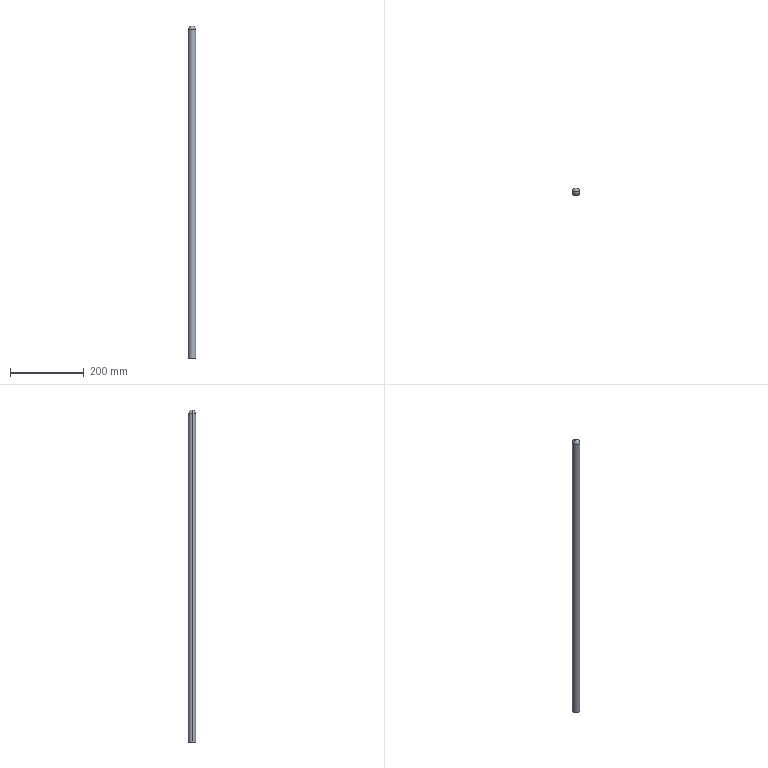Part | STEP file | X77-09003h | 1 solid | 6 faces | box 20 x 20 x 900 mm | volume 281698 mm3 | torus 2 | cylinder 2 | plane 2 | commonest cylinder face diameters 20 x2
STEP:
#1=CARTESIAN_POINT('',(-10.,0.,890.01));
#2=VERTEX_POINT('',#1);
#3=CARTESIAN_POINT('',(10.,0.,890.01));
#4=VERTEX_POINT('',#3);
#5=CARTESIAN_POINT('',(0.,0.,890.01));
#6=DIRECTION('',(0.,0.,-1.));
#7=DIRECTION('',(1.,0.,0.));
#8=AXIS2_PLACEMENT_3D('',#5,#6,#7);
#9=CIRCLE('',#8,10.);
#10=EDGE_CURVE('',#2,#4,#9,.T.);
#11=ORIENTED_EDGE('',*,*,#10,.F.);
#12=CARTESIAN_POINT('',(-0.01,0.,900.));
#13=VERTEX_POINT('',#12);
#14=CARTESIAN_POINT('',(-0.01,0.,890.01));
#15=DIRECTION('',(0.,1.,0.));
#16=DIRECTION('',(-1.,0.,0.));
#17=AXIS2_PLACEMENT_3D('',#14,#15,#16);
#18=CIRCLE('',#17,9.99);
#19=EDGE_CURVE('',#2,#13,#18,.T.);
#20=ORIENTED_EDGE('',*,*,#19,.T.);
#21=CARTESIAN_POINT('',(0.01,0.,900.));
#22=VERTEX_POINT('',#21);
#23=CARTESIAN_POINT('',(0.,0.,900.));
#24=DIRECTION('',(0.,0.,1.));
#25=DIRECTION('',(1.,0.,0.));
#26=AXIS2_PLACEMENT_3D('',#23,#24,#25);
#27=CIRCLE('',#26,0.01);
#28=EDGE_CURVE('',#22,#13,#27,.T.);
#29=ORIENTED_EDGE('',*,*,#28,.F.);
#30=CARTESIAN_POINT('',(0.01,0.,890.01));
#31=DIRECTION('',(0.,-1.,0.));
#32=DIRECTION('',(0.,0.,-1.));
#33=AXIS2_PLACEMENT_3D('',#30,#31,#32);
#34=CIRCLE('',#33,9.99);
#35=EDGE_CURVE('',#4,#22,#34,.T.);
#36=ORIENTED_EDGE('',*,*,#35,.F.);
#37=EDGE_LOOP('',(#11,#20,#29,#36));
#38=FACE_OUTER_BOUND('',#37,.T.);
#39=CARTESIAN_POINT('',(0.,0.,890.01));
#40=DIRECTION('',(0.,0.,1.));
#41=DIRECTION('',(1.,0.,0.));
#42=AXIS2_PLACEMENT_3D('',#39,#40,#41);
#43=TOROIDAL_SURFACE('',#42,0.01,9.99);
#44=ADVANCED_FACE('',(#38),#43,.T.);
#45=ORIENTED_EDGE('',*,*,#10,.T.);
#46=CARTESIAN_POINT('',(10.,0.,0.));
#47=VERTEX_POINT('',#46);
#48=CARTESIAN_POINT('',(10.,0.,900.));
#49=DIRECTION('',(0.,0.,-1.));
#50=VECTOR('',#49,1000.);
#51=LINE('',#48,#50);
#52=EDGE_CURVE('',#4,#47,#51,.T.);
#53=ORIENTED_EDGE('',*,*,#52,.T.);
#54=CARTESIAN_POINT('',(-10.,0.,0.));
#55=VERTEX_POINT('',#54);
#56=CARTESIAN_POINT('',(0.,0.,0.));
#57=DIRECTION('',(0.,0.,1.));
#58=DIRECTION('',(1.,0.,0.));
#59=AXIS2_PLACEMENT_3D('',#56,#57,#58);
#60=CIRCLE('',#59,10.);
#61=EDGE_CURVE('',#47,#55,#60,.T.);
#62=ORIENTED_EDGE('',*,*,#61,.T.);
#63=CARTESIAN_POINT('',(-10.,0.,900.));
#64=DIRECTION('',(0.,0.,-1.));
#65=VECTOR('',#64,1000.);
#66=LINE('',#63,#65);
#67=EDGE_CURVE('',#2,#55,#66,.T.);
#68=ORIENTED_EDGE('',*,*,#67,.F.);
#69=EDGE_LOOP('',(#45,#53,#62,#68));
#70=FACE_OUTER_BOUND('',#69,.T.);
#71=CARTESIAN_POINT('',(0.,0.,900.));
#72=DIRECTION('',(0.,0.,-1.));
#73=DIRECTION('',(-1.,0.,0.));
#74=AXIS2_PLACEMENT_3D('',#71,#72,#73);
#75=CYLINDRICAL_SURFACE('',#74,10.);
#76=ADVANCED_FACE('',(#70),#75,.T.);
#77=ORIENTED_EDGE('',*,*,#52,.F.);
#78=CARTESIAN_POINT('',(0.,0.,890.01));
#79=DIRECTION('',(0.,0.,-1.));
#80=DIRECTION('',(1.,0.,0.));
#81=AXIS2_PLACEMENT_3D('',#78,#79,#80);
#82=CIRCLE('',#81,10.);
#83=EDGE_CURVE('',#4,#2,#82,.T.);
#84=ORIENTED_EDGE('',*,*,#83,.T.);
#85=ORIENTED_EDGE('',*,*,#67,.T.);
#86=CARTESIAN_POINT('',(0.,0.,0.));
#87=DIRECTION('',(0.,0.,1.));
#88=DIRECTION('',(1.,0.,0.));
#89=AXIS2_PLACEMENT_3D('',#86,#87,#88);
#90=CIRCLE('',#89,10.);
#91=EDGE_CURVE('',#55,#47,#90,.T.);
#92=ORIENTED_EDGE('',*,*,#91,.T.);
#93=EDGE_LOOP('',(#77,#84,#85,#92));
#94=FACE_OUTER_BOUND('',#93,.T.);
#95=CARTESIAN_POINT('',(0.,0.,900.));
#96=DIRECTION('',(0.,0.,-1.));
#97=DIRECTION('',(-1.,0.,0.));
#98=AXIS2_PLACEMENT_3D('',#95,#96,#97);
#99=CYLINDRICAL_SURFACE('',#98,10.);
#100=ADVANCED_FACE('',(#94),#99,.T.);
#101=ORIENTED_EDGE('',*,*,#28,.T.);
#102=CARTESIAN_POINT('',(0.,0.,900.));
#103=DIRECTION('',(0.,0.,1.));
#104=DIRECTION('',(1.,0.,0.));
#105=AXIS2_PLACEMENT_3D('',#102,#103,#104);
#106=CIRCLE('',#105,0.01);
#107=EDGE_CURVE('',#13,#22,#106,.T.);
#108=ORIENTED_EDGE('',*,*,#107,.T.);
#109=EDGE_LOOP('',(#101,#108));
#110=FACE_OUTER_BOUND('',#109,.T.);
#111=CARTESIAN_POINT('',(0.,0.,900.));
#112=DIRECTION('',(0.,0.,1.));
#113=DIRECTION('',(1.,0.,0.));
#114=AXIS2_PLACEMENT_3D('',#111,#112,#113);
#115=PLANE('',#114);
#116=ADVANCED_FACE('',(#110),#115,.T.);
#117=ORIENTED_EDGE('',*,*,#91,.F.);
#118=ORIENTED_EDGE('',*,*,#61,.F.);
#119=EDGE_LOOP('',(#117,#118));
#120=FACE_OUTER_BOUND('',#119,.T.);
#121=CARTESIAN_POINT('',(0.,0.,0.));
#122=DIRECTION('',(0.,0.,1.));
#123=DIRECTION('',(1.,0.,0.));
#124=AXIS2_PLACEMENT_3D('',#121,#122,#123);
#125=PLANE('',#124);
#126=ADVANCED_FACE('',(#120),#125,.F.);
#127=ORIENTED_EDGE('',*,*,#19,.F.);
#128=ORIENTED_EDGE('',*,*,#83,.F.);
#129=ORIENTED_EDGE('',*,*,#35,.T.);
#130=ORIENTED_EDGE('',*,*,#107,.F.);
#131=EDGE_LOOP('',(#127,#128,#129,#130));
#132=FACE_OUTER_BOUND('',#131,.T.);
#133=CARTESIAN_POINT('',(0.,0.,890.01));
#134=DIRECTION('',(0.,0.,1.));
#135=DIRECTION('',(1.,0.,0.));
#136=AXIS2_PLACEMENT_3D('',#133,#134,#135);
#137=TOROIDAL_SURFACE('',#136,0.01,9.99);
#138=ADVANCED_FACE('',(#132),#137,.T.);
#139=CLOSED_SHELL('',(#44,#76,#100,#116,#126,#138));
#140=MANIFOLD_SOLID_BREP('',#139);
#141=CARTESIAN_POINT('',(0.,0.,0.));
#142=DIRECTION('',(0.,0.,1.));
#143=DIRECTION('',(1.,0.,0.));
#144=AXIS2_PLACEMENT_3D('',#141,#142,#143);
#145=(LENGTH_UNIT()NAMED_UNIT(*)SI_UNIT(.MILLI.,.METRE.));
#146=UNCERTAINTY_MEASURE_WITH_UNIT(LENGTH_MEASURE(0.00001),#145,'','');
#147=(NAMED_UNIT(*)PLANE_ANGLE_UNIT()SI_UNIT($,.RADIAN.));
#148=(NAMED_UNIT(*)SI_UNIT($,.STERADIAN.)SOLID_ANGLE_UNIT());
#149=(GEOMETRIC_REPRESENTATION_CONTEXT(3)GLOBAL_UNCERTAINTY_ASSIGNED_CONTEXT((#146))GLOBAL_UNIT_ASSIGNED_CONTEXT((#145,#147,#148))REPRESENTATION_CONTEXT('',''));
#150=ADVANCED_BREP_SHAPE_REPRESENTATION('',(#140,#144),#149);